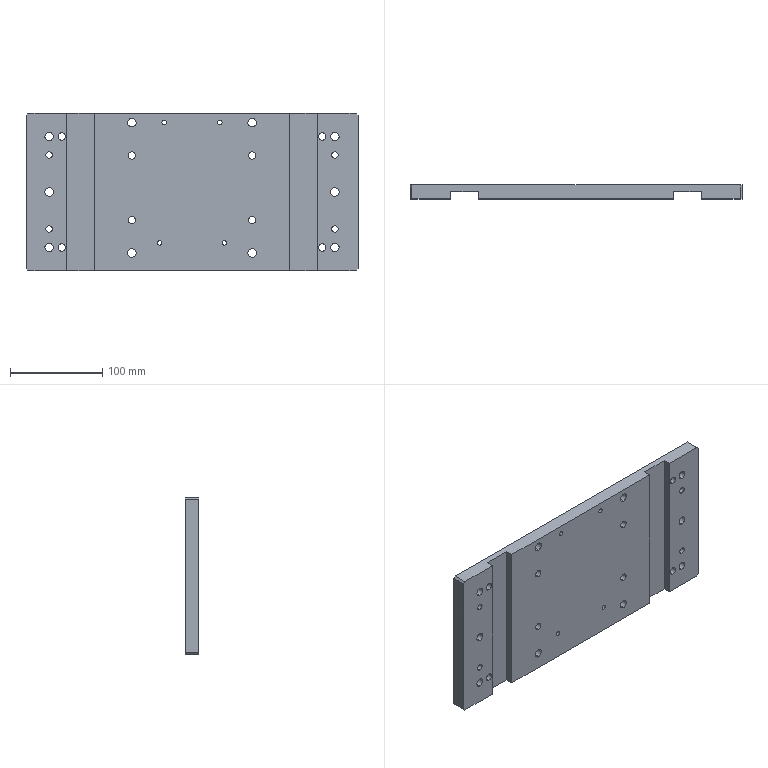Part | STEP file | PN_0016_default | 1 solid | 120 faces | box 359 x 15 x 170 mm | volume 803822 mm3 | cylinder 82 | plane 28 | cone 10 | commonest cylinder face diameters 9 x20 15 x20 5 x18 8 x16 6.8 x8